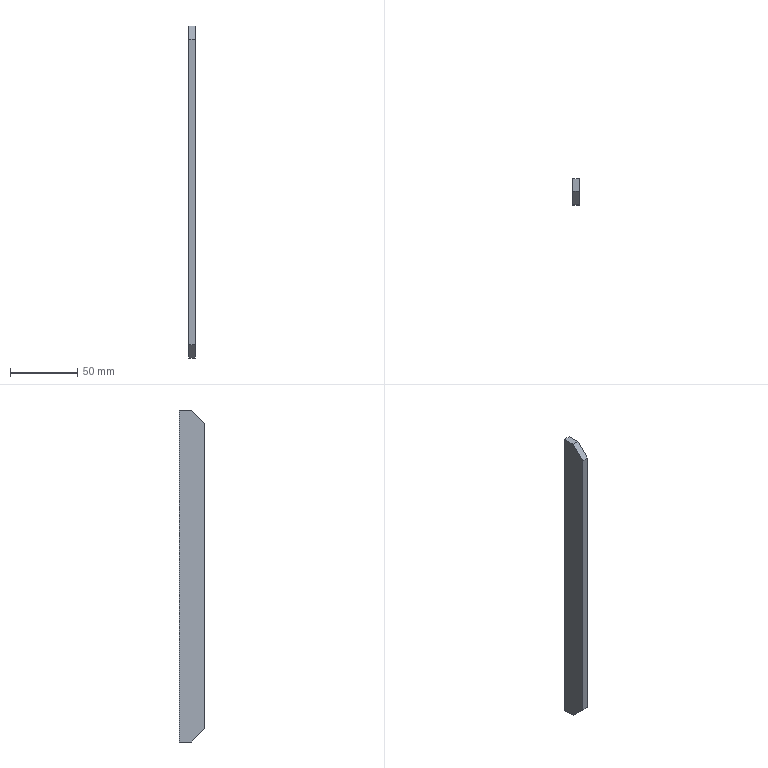Part | SolidWorks | features 3DProfileFeature 1, Chamfer 1, Extrusion 1 | 1 solid | 8 faces | box 5 x 19 x 247 mm | volume 22965 mm3 | plane 8
STEP:
#1=CARTESIAN_POINT('',(2.5,0.5,-123.5));
#2=VERTEX_POINT('',#1);
#3=CARTESIAN_POINT('',(2.5,9.5,-123.5));
#4=VERTEX_POINT('',#3);
#5=CARTESIAN_POINT('',(2.5,-9.5,-123.5));
#6=DIRECTION('',(0.,1.,0.));
#7=VECTOR('',#6,1000.);
#8=LINE('',#5,#7);
#9=EDGE_CURVE('',#2,#4,#8,.T.);
#10=ORIENTED_EDGE('',*,*,#9,.F.);
#11=CARTESIAN_POINT('',(-2.5,0.5,-123.5));
#12=VERTEX_POINT('',#11);
#13=CARTESIAN_POINT('',(2.5,0.5,-123.5));
#14=DIRECTION('',(-1.,0.,0.));
#15=VECTOR('',#14,1000.);
#16=LINE('',#13,#15);
#17=EDGE_CURVE('',#2,#12,#16,.T.);
#18=ORIENTED_EDGE('',*,*,#17,.T.);
#19=CARTESIAN_POINT('',(-2.5,9.5,-123.5));
#20=VERTEX_POINT('',#19);
#21=CARTESIAN_POINT('',(-2.5,-9.5,-123.5));
#22=DIRECTION('',(0.,1.,0.));
#23=VECTOR('',#22,1000.);
#24=LINE('',#21,#23);
#25=EDGE_CURVE('',#12,#20,#24,.T.);
#26=ORIENTED_EDGE('',*,*,#25,.T.);
#27=CARTESIAN_POINT('',(2.5,9.5,-123.5));
#28=DIRECTION('',(-1.,0.,0.));
#29=VECTOR('',#28,1000.);
#30=LINE('',#27,#29);
#31=EDGE_CURVE('',#4,#20,#30,.T.);
#32=ORIENTED_EDGE('',*,*,#31,.F.);
#33=EDGE_LOOP('',(#10,#18,#26,#32));
#34=FACE_OUTER_BOUND('',#33,.T.);
#35=CARTESIAN_POINT('',(2.5,-9.5,-123.5));
#36=DIRECTION('',(0.,0.,1.));
#37=DIRECTION('',(1.,0.,0.));
#38=AXIS2_PLACEMENT_3D('',#35,#36,#37);
#39=PLANE('',#38);
#40=ADVANCED_FACE('',(#34),#39,.F.);
#41=CARTESIAN_POINT('',(-2.5,9.5,123.5));
#42=VERTEX_POINT('',#41);
#43=CARTESIAN_POINT('',(-2.5,9.5,123.5));
#44=DIRECTION('',(0.,0.,1.));
#45=VECTOR('',#44,1000.);
#46=LINE('',#43,#45);
#47=EDGE_CURVE('',#20,#42,#46,.T.);
#48=ORIENTED_EDGE('',*,*,#47,.T.);
#49=CARTESIAN_POINT('',(2.5,9.5,123.5));
#50=VERTEX_POINT('',#49);
#51=CARTESIAN_POINT('',(2.5,9.5,123.5));
#52=DIRECTION('',(-1.,0.,0.));
#53=VECTOR('',#52,1000.);
#54=LINE('',#51,#53);
#55=EDGE_CURVE('',#50,#42,#54,.T.);
#56=ORIENTED_EDGE('',*,*,#55,.F.);
#57=CARTESIAN_POINT('',(2.5,9.5,123.5));
#58=DIRECTION('',(0.,0.,1.));
#59=VECTOR('',#58,1000.);
#60=LINE('',#57,#59);
#61=EDGE_CURVE('',#4,#50,#60,.T.);
#62=ORIENTED_EDGE('',*,*,#61,.F.);
#63=ORIENTED_EDGE('',*,*,#31,.T.);
#64=EDGE_LOOP('',(#48,#56,#62,#63));
#65=FACE_OUTER_BOUND('',#64,.T.);
#66=CARTESIAN_POINT('',(2.5,9.5,123.5));
#67=DIRECTION('',(0.,-1.,0.));
#68=DIRECTION('',(0.,0.,-1.));
#69=AXIS2_PLACEMENT_3D('',#66,#67,#68);
#70=PLANE('',#69);
#71=ADVANCED_FACE('',(#65),#70,.F.);
#72=CARTESIAN_POINT('',(-2.5,0.5,123.5));
#73=VERTEX_POINT('',#72);
#74=CARTESIAN_POINT('',(-2.5,-9.5,123.5));
#75=DIRECTION('',(0.,-1.,0.));
#76=VECTOR('',#75,1000.);
#77=LINE('',#74,#76);
#78=EDGE_CURVE('',#42,#73,#77,.T.);
#79=ORIENTED_EDGE('',*,*,#78,.T.);
#80=CARTESIAN_POINT('',(2.5,0.5,123.5));
#81=VERTEX_POINT('',#80);
#82=CARTESIAN_POINT('',(2.5,0.5,123.5));
#83=DIRECTION('',(1.,0.,0.));
#84=VECTOR('',#83,1000.);
#85=LINE('',#82,#84);
#86=EDGE_CURVE('',#73,#81,#85,.T.);
#87=ORIENTED_EDGE('',*,*,#86,.T.);
#88=CARTESIAN_POINT('',(2.5,-9.5,123.5));
#89=DIRECTION('',(0.,-1.,0.));
#90=VECTOR('',#89,1000.);
#91=LINE('',#88,#90);
#92=EDGE_CURVE('',#50,#81,#91,.T.);
#93=ORIENTED_EDGE('',*,*,#92,.F.);
#94=ORIENTED_EDGE('',*,*,#55,.T.);
#95=EDGE_LOOP('',(#79,#87,#93,#94));
#96=FACE_OUTER_BOUND('',#95,.T.);
#97=CARTESIAN_POINT('',(2.5,-9.5,123.5));
#98=DIRECTION('',(0.,0.,-1.));
#99=DIRECTION('',(-1.,0.,0.));
#100=AXIS2_PLACEMENT_3D('',#97,#98,#99);
#101=PLANE('',#100);
#102=ADVANCED_FACE('',(#96),#101,.F.);
#103=CARTESIAN_POINT('',(-2.5,-9.5,113.5));
#104=VERTEX_POINT('',#103);
#105=CARTESIAN_POINT('',(-2.5,-9.5,-113.5));
#106=VERTEX_POINT('',#105);
#107=CARTESIAN_POINT('',(-2.5,-9.5,123.5));
#108=DIRECTION('',(0.,0.,-1.));
#109=VECTOR('',#108,1000.);
#110=LINE('',#107,#109);
#111=EDGE_CURVE('',#104,#106,#110,.T.);
#112=ORIENTED_EDGE('',*,*,#111,.T.);
#113=CARTESIAN_POINT('',(2.5,-9.5,-113.5));
#114=VERTEX_POINT('',#113);
#115=CARTESIAN_POINT('',(2.5,-9.5,-113.5));
#116=DIRECTION('',(1.,0.,0.));
#117=VECTOR('',#116,1000.);
#118=LINE('',#115,#117);
#119=EDGE_CURVE('',#106,#114,#118,.T.);
#120=ORIENTED_EDGE('',*,*,#119,.T.);
#121=CARTESIAN_POINT('',(2.5,-9.5,113.5));
#122=VERTEX_POINT('',#121);
#123=CARTESIAN_POINT('',(2.5,-9.5,123.5));
#124=DIRECTION('',(0.,0.,-1.));
#125=VECTOR('',#124,1000.);
#126=LINE('',#123,#125);
#127=EDGE_CURVE('',#122,#114,#126,.T.);
#128=ORIENTED_EDGE('',*,*,#127,.F.);
#129=CARTESIAN_POINT('',(2.5,-9.5,113.5));
#130=DIRECTION('',(-1.,0.,0.));
#131=VECTOR('',#130,1000.);
#132=LINE('',#129,#131);
#133=EDGE_CURVE('',#122,#104,#132,.T.);
#134=ORIENTED_EDGE('',*,*,#133,.T.);
#135=EDGE_LOOP('',(#112,#120,#128,#134));
#136=FACE_OUTER_BOUND('',#135,.T.);
#137=CARTESIAN_POINT('',(2.5,-9.5,123.5));
#138=DIRECTION('',(0.,1.,0.));
#139=DIRECTION('',(0.,0.,1.));
#140=AXIS2_PLACEMENT_3D('',#137,#138,#139);
#141=PLANE('',#140);
#142=ADVANCED_FACE('',(#136),#141,.F.);
#143=ORIENTED_EDGE('',*,*,#127,.T.);
#144=CARTESIAN_POINT('',(2.5,0.5,-123.5));
#145=DIRECTION('',(0.,0.7071,-0.7071));
#146=VECTOR('',#145,1000.);
#147=LINE('',#144,#146);
#148=EDGE_CURVE('',#114,#2,#147,.T.);
#149=ORIENTED_EDGE('',*,*,#148,.T.);
#150=ORIENTED_EDGE('',*,*,#9,.T.);
#151=ORIENTED_EDGE('',*,*,#61,.T.);
#152=ORIENTED_EDGE('',*,*,#92,.T.);
#153=CARTESIAN_POINT('',(2.5,-9.5,113.5));
#154=DIRECTION('',(0.,-0.7071,-0.7071));
#155=VECTOR('',#154,1000.);
#156=LINE('',#153,#155);
#157=EDGE_CURVE('',#81,#122,#156,.T.);
#158=ORIENTED_EDGE('',*,*,#157,.T.);
#159=EDGE_LOOP('',(#143,#149,#150,#151,#152,#158));
#160=FACE_OUTER_BOUND('',#159,.T.);
#161=CARTESIAN_POINT('',(2.5,0.,0.));
#162=DIRECTION('',(-1.,0.,0.));
#163=DIRECTION('',(0.,0.,1.));
#164=AXIS2_PLACEMENT_3D('',#161,#162,#163);
#165=PLANE('',#164);
#166=ADVANCED_FACE('',(#160),#165,.F.);
#167=ORIENTED_EDGE('',*,*,#25,.F.);
#168=CARTESIAN_POINT('',(-2.5,-61.5,-61.5));
#169=DIRECTION('',(0.,-0.7071,0.7071));
#170=VECTOR('',#169,1000.);
#171=LINE('',#168,#170);
#172=EDGE_CURVE('',#12,#106,#171,.T.);
#173=ORIENTED_EDGE('',*,*,#172,.T.);
#174=ORIENTED_EDGE('',*,*,#111,.F.);
#175=CARTESIAN_POINT('',(-2.5,-61.5,61.5));
#176=DIRECTION('',(0.,0.7071,0.7071));
#177=VECTOR('',#176,1000.);
#178=LINE('',#175,#177);
#179=EDGE_CURVE('',#104,#73,#178,.T.);
#180=ORIENTED_EDGE('',*,*,#179,.T.);
#181=ORIENTED_EDGE('',*,*,#78,.F.);
#182=ORIENTED_EDGE('',*,*,#47,.F.);
#183=EDGE_LOOP('',(#167,#173,#174,#180,#181,#182));
#184=FACE_OUTER_BOUND('',#183,.T.);
#185=CARTESIAN_POINT('',(-2.5,0.,0.));
#186=DIRECTION('',(-1.,0.,0.));
#187=DIRECTION('',(0.,0.,1.));
#188=AXIS2_PLACEMENT_3D('',#185,#186,#187);
#189=PLANE('',#188);
#190=ADVANCED_FACE('',(#184),#189,.T.);
#191=ORIENTED_EDGE('',*,*,#148,.F.);
#192=ORIENTED_EDGE('',*,*,#119,.F.);
#193=ORIENTED_EDGE('',*,*,#172,.F.);
#194=ORIENTED_EDGE('',*,*,#17,.F.);
#195=EDGE_LOOP('',(#191,#192,#193,#194));
#196=FACE_OUTER_BOUND('',#195,.T.);
#197=CARTESIAN_POINT('',(2.5,0.5,-123.5));
#198=DIRECTION('',(0.,0.7071,0.7071));
#199=DIRECTION('',(-1.,0.,0.));
#200=AXIS2_PLACEMENT_3D('',#197,#198,#199);
#201=PLANE('',#200);
#202=ADVANCED_FACE('',(#196),#201,.F.);
#203=ORIENTED_EDGE('',*,*,#157,.F.);
#204=ORIENTED_EDGE('',*,*,#86,.F.);
#205=ORIENTED_EDGE('',*,*,#179,.F.);
#206=ORIENTED_EDGE('',*,*,#133,.F.);
#207=EDGE_LOOP('',(#203,#204,#205,#206));
#208=FACE_OUTER_BOUND('',#207,.T.);
#209=CARTESIAN_POINT('',(2.5,-9.5,113.5));
#210=DIRECTION('',(0.,0.7071,-0.7071));
#211=DIRECTION('',(-1.,0.,0.));
#212=AXIS2_PLACEMENT_3D('',#209,#210,#211);
#213=PLANE('',#212);
#214=ADVANCED_FACE('',(#208),#213,.F.);
#215=CLOSED_SHELL('',(#40,#71,#102,#142,#166,#190,#202,#214));
#216=MANIFOLD_SOLID_BREP('',#215);
#217=CARTESIAN_POINT('',(0.,0.,0.));
#218=DIRECTION('',(0.,0.,1.));
#219=DIRECTION('',(1.,0.,0.));
#220=AXIS2_PLACEMENT_3D('',#217,#218,#219);
#221=(LENGTH_UNIT()NAMED_UNIT(*)SI_UNIT(.MILLI.,.METRE.));
#222=UNCERTAINTY_MEASURE_WITH_UNIT(LENGTH_MEASURE(0.00001),#221,'','');
#223=(NAMED_UNIT(*)PLANE_ANGLE_UNIT()SI_UNIT($,.RADIAN.));
#224=(NAMED_UNIT(*)SI_UNIT($,.STERADIAN.)SOLID_ANGLE_UNIT());
#225=(GEOMETRIC_REPRESENTATION_CONTEXT(3)GLOBAL_UNCERTAINTY_ASSIGNED_CONTEXT((#222))GLOBAL_UNIT_ASSIGNED_CONTEXT((#221,#223,#224))REPRESENTATION_CONTEXT('',''));
#226=ADVANCED_BREP_SHAPE_REPRESENTATION('',(#216,#220),#225);